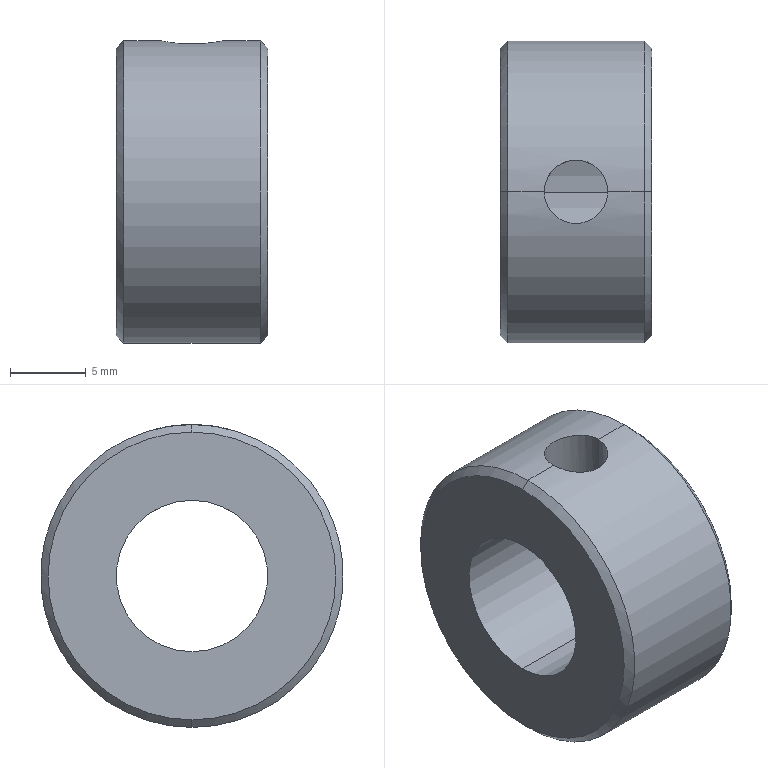Part | STEP file | 8XS210011 | 1 solid | 12 faces | box 10 x 20 x 20 mm | volume 2271 mm3 | cylinder 6 | cone 4 | plane 2 | commonest cylinder face diameters 4.2 x2 10 x2 20 x2